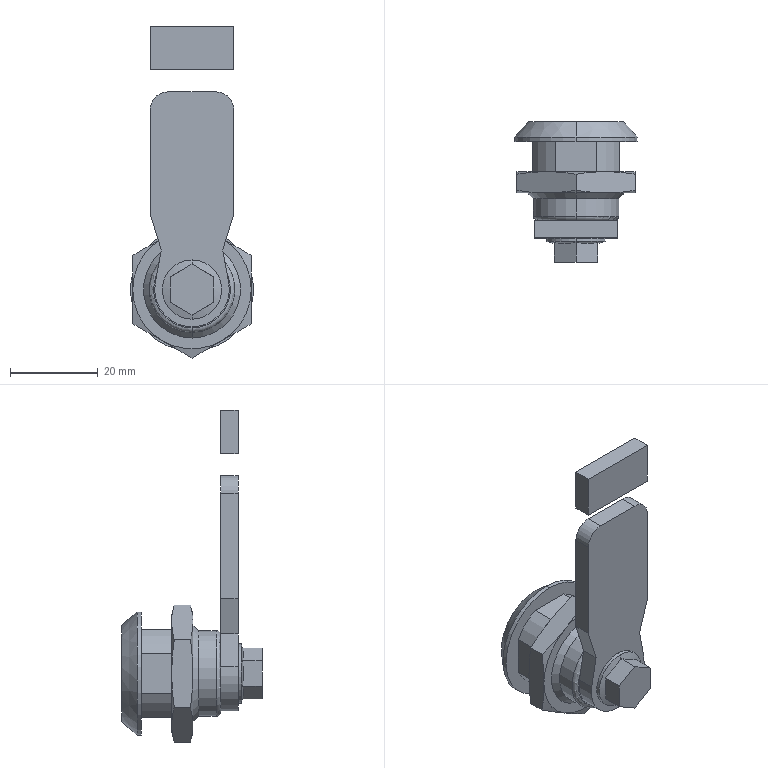Part | SolidWorks | features BaseBody 1, ICE 1, MoveCopyBody 1, Split 1 | 2 solids | 85 faces | box 28 x 32 x 75.588 mm | volume 13581 mm3 | plane 42 | cone 20 | cylinder 19 | torus 4 | commonest cylinder face diameters 9.5 x4 22 x4 8 x2 13.5 x2 16.1 x2 19.5 x2